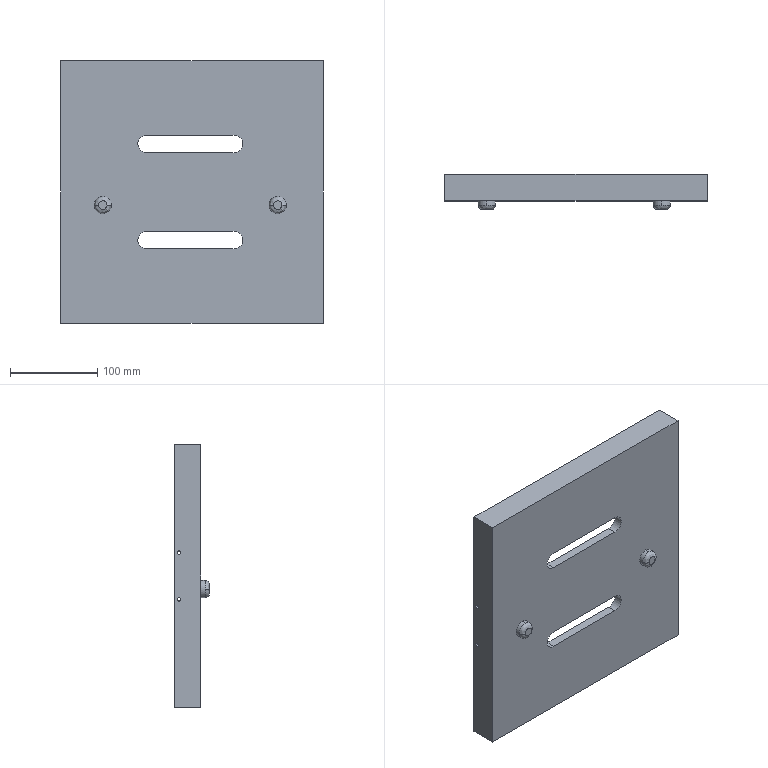Part | STEP file | leg control02_5 | 1 solid | 37 faces | box 300 x 40 x 300 mm | volume 1254281 mm3 | plane 17 | cylinder 16 | spline 4 | commonest cylinder face diameters 4 x8 19.8 x4 20 x4